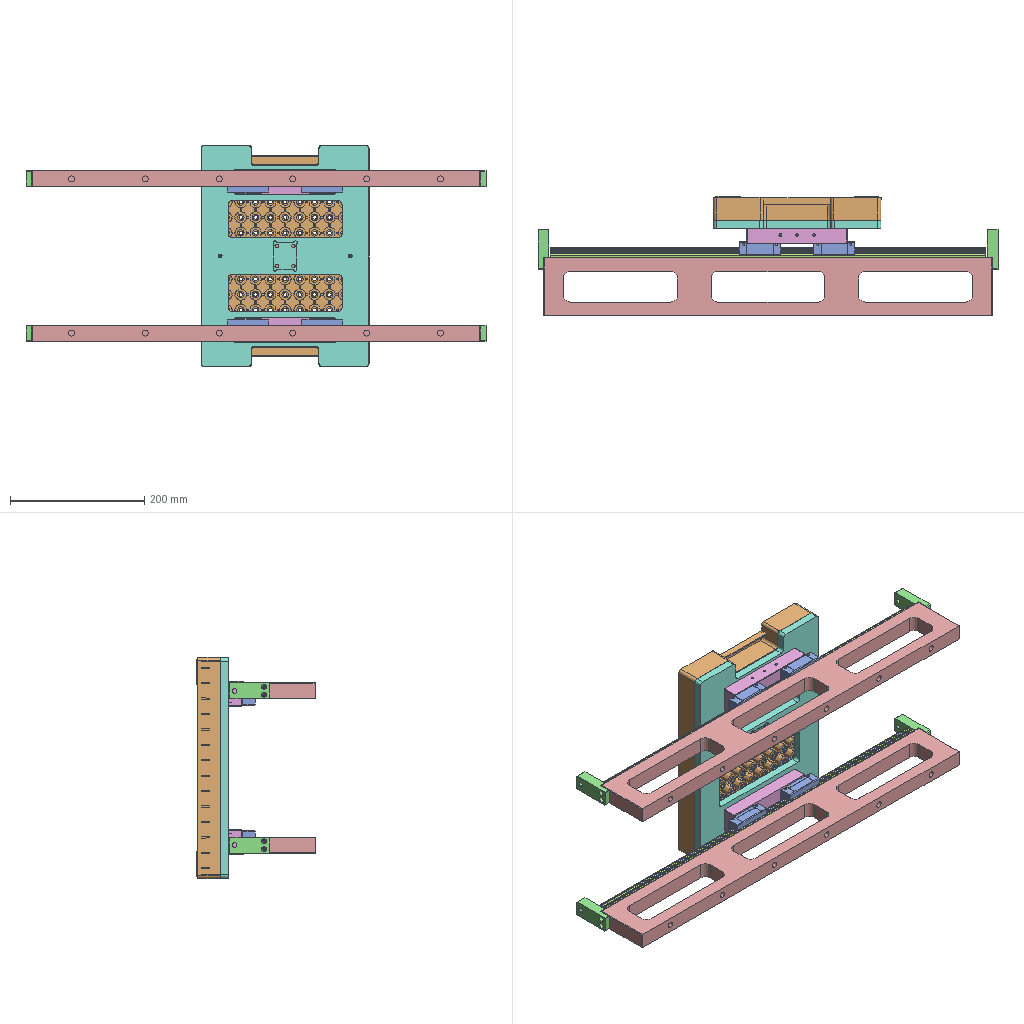Assembly | SolidWorks | 9 different items | 20 placed | box 686 x 178 x 330 mm
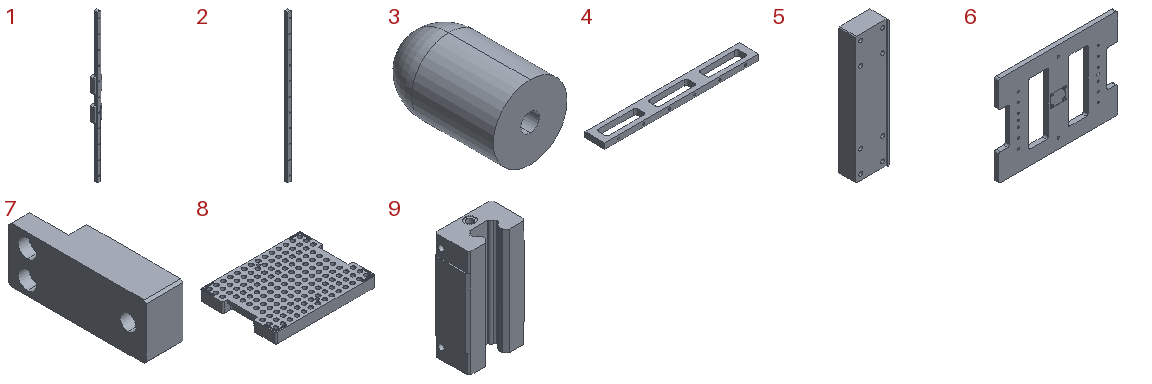Parts list (item | name | quantity | parent item | size | volume | features):
1 | (subassembly) | x2 | - | 34 x 24 x 650 mm | 182322 mm3 | -
2 | - | x2 | in 1 | 15 x 15 x 650 mm | 119721 mm3 | features MoveFace 2, BaseBody 1, LPattern 1
3 | - | x2 | - | 9.95 x 15.5 x 9.95 mm | 1091 mm3 | features HoleWzd 1, Revolution 1
4 | - | x2 | - | 670 x 86 x 24 mm | 815923 mm3 | features HoleWzd 5, Chamfer 1, Extrusion 1, ICE 1
5 | - | x2 | - | 38 x 22 x 150 mm | 108993 mm3 | features HoleWzd 4, Chamfer 1, Extrusion 1
6 | - | x1 | - | 329 x 12 x 250 mm | 676996 mm3 | features HoleWzd 5, ICE 4, Fillet 3, Extrusion 1
7 | - | x4 | - | 16 x 60 x 24 mm | 18592 mm3 | features BaseBody 1, Chamfer 1, HoleWzd 1, ICE 1
8 | - | x1 | - | - | 715592 mm3 | features BaseBody 1
9 | - | x4 | in 1 | 34 x 19.7 x 61.4 mm | 31300 mm3 | features BaseBody 1
Mates (type | each side: item.copy, entity, surface, feature):
In the top assembly
Coincident | 4.1 face plane Boss-Extrude1 | 2.1 face plane Input1
Concentric | 4.1 face cylinder M4 Tapped Hole1 | 2.1 face cylinder Input1
Parallel | 4.1 face plane Boss-Extrude1 | 2.1 face plane Input1
Concentric | 2.2 face cylinder Input1 | 4.2 face cylinder M4 Tapped Hole1
Coincident | 2.2 face plane Input1 | 4.2 face plane Boss-Extrude1
Parallel | 2.2 face plane Input1 | 4.2 face plane Boss-Extrude1
Coincident | 4.1 face plane Boss-Extrude1 | 4.2 face plane Boss-Extrude1 | 2 times
DistanceDim | 4.2 face plane Boss-Extrude1 | 4.1 face plane Boss-Extrude1
Coincident | 9.1 face plane Input1 | 5.1 face plane Boss-Extrude1 | 3 times
Coincident | 9.2 face plane Input1 | 5.2 face plane Boss-Extrude1 | 3 times
Coincident | 9.1 face plane Input1 | 9.3 face plane Input1
Coincident | 5.2 face plane Boss-Extrude1 | 6.1 face plane Boss-Extrude1
Width | 6.1 face plane Boss-Extrude1 | 6.1 face plane Boss-Extrude1 | 5.1 face plane Boss-Extrude1 | 5.1 face plane Boss-Extrude1
Width | 6.1 face plane Boss-Extrude1 | 6.1 face plane Boss-Extrude1 | 5.2 face plane Boss-Extrude1 | 5.1 face plane Boss-Extrude1
Concentric | 6.1 face cylinder Cut-Extrude1 | 8.1 face cylinder Input1 | 2 times
Coincident | 6.1 face plane Boss-Extrude1 | 8.1 face plane Input1
Concentric | 6.1 face cylinder Cut-Extrude1 | 3.1 face cylinder Revolve1
Coincident | 6.1 face plane Cut-Extrude1 | 3.1 face plane Revolve1
Coincident | 6.1 face plane Cut-Extrude1 | 3.2 face plane Revolve1
Concentric | 6.1 face cylinder Cut-Extrude1 | 3.2 face cylinder Revolve1
Coincident | 4.2 face plane Boss-Extrude1 | 7.1 face plane Input1
Coincident | 4.2 face plane Boss-Extrude1 | 7.2 face plane Input1
Concentric | 4.2 face cylinder M4 Tapped Hole3 | 7.1 face cylinder Input1 | 2 times
Concentric | 4.2 face cylinder M4 Tapped Hole2 | 7.2 face cylinder Input1 | 2 times
In subassembly 1
Coincident | 9.4 face plane Input1 | 2.3 face plane Input1
Width | 9.4 face plane Input1 | 9.4 face plane Input1 | 2.3 face plane Input1 | 2.3 face plane Input1
Coincident | 2.3 face plane Input1 | 9.5 face plane Input1
Width | 9.5 face plane Input1 | 9.5 face plane Input1 | 2.3 face plane Input1 | 2.3 face plane Input1
LimitDistanceDim | 9.4 face plane Input1 | 2.3 face plane Input1
LimitDistanceDim | 9.5 face plane Input1 | 2.3 face plane Input1
DistanceDim | 9.4 face plane Input1 | 9.5 face plane Input1